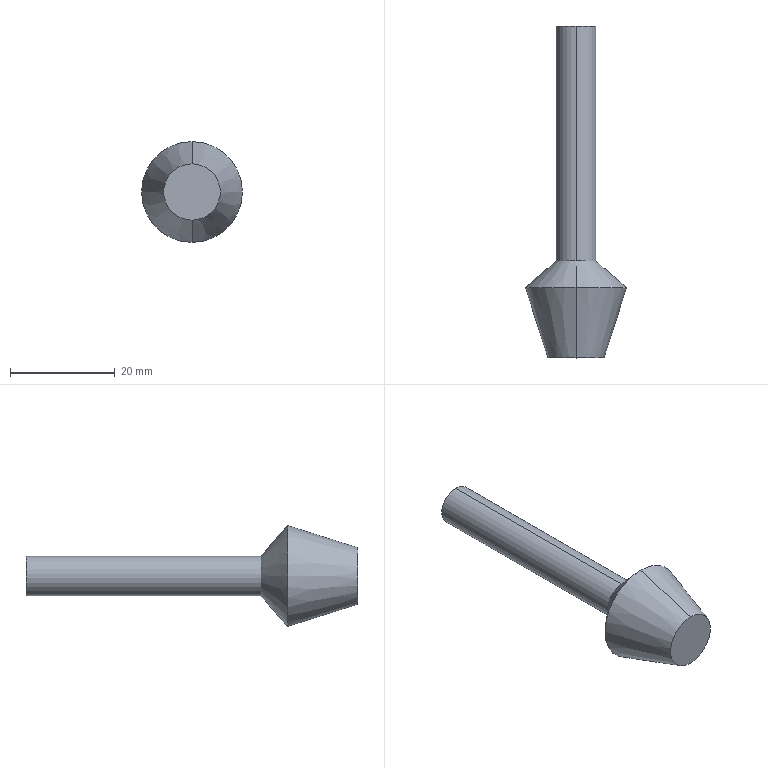Part | SolidWorks | features Revolution 1 | 1 solid | 8 faces | box 19.304 x 63.5 x 19.304 mm | volume 5277 mm3 | cone 4 | cylinder 2 | plane 2 | commonest cylinder face diameters 7.62 x2
STEP:
#1=CARTESIAN_POINT('',(0.,0.,-0.2125));
#2=VERTEX_POINT('',#1);
#3=CARTESIAN_POINT('',(0.,0.,0.2125));
#4=VERTEX_POINT('',#3);
#5=CARTESIAN_POINT('',(0.,0.,0.));
#6=DIRECTION('',(0.,-1.,0.));
#7=DIRECTION('',(0.,0.,-1.));
#8=AXIS2_PLACEMENT_3D('',#5,#6,#7);
#9=CIRCLE('',#8,0.2125);
#10=EDGE_CURVE('',#2,#4,#9,.T.);
#11=ORIENTED_EDGE('',*,*,#10,.F.);
#12=CARTESIAN_POINT('',(0.,0.53,-0.38));
#13=VERTEX_POINT('',#12);
#14=CARTESIAN_POINT('',(0.,0.53,-0.38));
#15=DIRECTION('',(0.,0.9535,-0.3013));
#16=VECTOR('',#15,39.37);
#17=LINE('',#14,#16);
#18=EDGE_CURVE('',#2,#13,#17,.T.);
#19=ORIENTED_EDGE('',*,*,#18,.T.);
#20=CARTESIAN_POINT('',(0.,0.53,0.38));
#21=VERTEX_POINT('',#20);
#22=CARTESIAN_POINT('',(0.,0.53,0.));
#23=DIRECTION('',(0.,-1.,0.));
#24=DIRECTION('',(0.,0.,-1.));
#25=AXIS2_PLACEMENT_3D('',#22,#23,#24);
#26=CIRCLE('',#25,0.38);
#27=EDGE_CURVE('',#13,#21,#26,.T.);
#28=ORIENTED_EDGE('',*,*,#27,.T.);
#29=CARTESIAN_POINT('',(0.,0.53,0.38));
#30=DIRECTION('',(0.,0.9535,0.3013));
#31=VECTOR('',#30,39.37);
#32=LINE('',#29,#31);
#33=EDGE_CURVE('',#4,#21,#32,.T.);
#34=ORIENTED_EDGE('',*,*,#33,.F.);
#35=EDGE_LOOP('',(#11,#19,#28,#34));
#36=FACE_OUTER_BOUND('',#35,.T.);
#37=CARTESIAN_POINT('',(0.,0.53,0.));
#38=DIRECTION('',(0.,1.,0.));
#39=DIRECTION('',(0.,0.,1.));
#40=AXIS2_PLACEMENT_3D('',#37,#38,#39);
#41=CONICAL_SURFACE('',#40,0.38,0.3061);
#42=ADVANCED_FACE('',(#36),#41,.T.);
#43=CARTESIAN_POINT('',(0.,2.5,-0.15));
#44=VERTEX_POINT('',#43);
#45=CARTESIAN_POINT('',(0.,2.5,0.15));
#46=VERTEX_POINT('',#45);
#47=CARTESIAN_POINT('',(0.,2.5,0.));
#48=DIRECTION('',(0.,-1.,0.));
#49=DIRECTION('',(0.,0.,-1.));
#50=AXIS2_PLACEMENT_3D('',#47,#48,#49);
#51=CIRCLE('',#50,0.15);
#52=EDGE_CURVE('',#44,#46,#51,.T.);
#53=ORIENTED_EDGE('',*,*,#52,.T.);
#54=CARTESIAN_POINT('',(0.,0.73,0.15));
#55=VERTEX_POINT('',#54);
#56=CARTESIAN_POINT('',(0.,0.,0.15));
#57=DIRECTION('',(0.,-1.,0.));
#58=VECTOR('',#57,39.37);
#59=LINE('',#56,#58);
#60=EDGE_CURVE('',#46,#55,#59,.T.);
#61=ORIENTED_EDGE('',*,*,#60,.T.);
#62=CARTESIAN_POINT('',(0.,0.73,-0.15));
#63=VERTEX_POINT('',#62);
#64=CARTESIAN_POINT('',(0.,0.73,0.));
#65=DIRECTION('',(0.,-1.,0.));
#66=DIRECTION('',(0.,0.,-1.));
#67=AXIS2_PLACEMENT_3D('',#64,#65,#66);
#68=CIRCLE('',#67,0.15);
#69=EDGE_CURVE('',#63,#55,#68,.T.);
#70=ORIENTED_EDGE('',*,*,#69,.F.);
#71=CARTESIAN_POINT('',(0.,0.,-0.15));
#72=DIRECTION('',(0.,-1.,0.));
#73=VECTOR('',#72,39.37);
#74=LINE('',#71,#73);
#75=EDGE_CURVE('',#44,#63,#74,.T.);
#76=ORIENTED_EDGE('',*,*,#75,.F.);
#77=EDGE_LOOP('',(#53,#61,#70,#76));
#78=FACE_OUTER_BOUND('',#77,.T.);
#79=CARTESIAN_POINT('',(0.,0.,0.));
#80=DIRECTION('',(0.,-1.,0.));
#81=DIRECTION('',(0.,0.,-1.));
#82=AXIS2_PLACEMENT_3D('',#79,#80,#81);
#83=CYLINDRICAL_SURFACE('',#82,0.15);
#84=ADVANCED_FACE('',(#78),#83,.T.);
#85=ORIENTED_EDGE('',*,*,#69,.T.);
#86=CARTESIAN_POINT('',(0.,0.53,0.38));
#87=DIRECTION('',(0.,-0.6562,0.7546));
#88=VECTOR('',#87,39.37);
#89=LINE('',#86,#88);
#90=EDGE_CURVE('',#55,#21,#89,.T.);
#91=ORIENTED_EDGE('',*,*,#90,.T.);
#92=ORIENTED_EDGE('',*,*,#27,.F.);
#93=CARTESIAN_POINT('',(0.,0.53,-0.38));
#94=DIRECTION('',(0.,-0.6562,-0.7546));
#95=VECTOR('',#94,39.37);
#96=LINE('',#93,#95);
#97=EDGE_CURVE('',#63,#13,#96,.T.);
#98=ORIENTED_EDGE('',*,*,#97,.F.);
#99=EDGE_LOOP('',(#85,#91,#92,#98));
#100=FACE_OUTER_BOUND('',#99,.T.);
#101=CARTESIAN_POINT('',(0.,0.53,0.));
#102=DIRECTION('',(0.,-1.,0.));
#103=DIRECTION('',(0.,0.,-1.));
#104=AXIS2_PLACEMENT_3D('',#101,#102,#103);
#105=CONICAL_SURFACE('',#104,0.38,0.8551);
#106=ADVANCED_FACE('',(#100),#105,.T.);
#107=ORIENTED_EDGE('',*,*,#90,.F.);
#108=CARTESIAN_POINT('',(0.,0.73,0.));
#109=DIRECTION('',(0.,-1.,0.));
#110=DIRECTION('',(0.,0.,-1.));
#111=AXIS2_PLACEMENT_3D('',#108,#109,#110);
#112=CIRCLE('',#111,0.15);
#113=EDGE_CURVE('',#55,#63,#112,.T.);
#114=ORIENTED_EDGE('',*,*,#113,.T.);
#115=ORIENTED_EDGE('',*,*,#97,.T.);
#116=CARTESIAN_POINT('',(0.,0.53,0.));
#117=DIRECTION('',(0.,-1.,0.));
#118=DIRECTION('',(0.,0.,-1.));
#119=AXIS2_PLACEMENT_3D('',#116,#117,#118);
#120=CIRCLE('',#119,0.38);
#121=EDGE_CURVE('',#21,#13,#120,.T.);
#122=ORIENTED_EDGE('',*,*,#121,.F.);
#123=EDGE_LOOP('',(#107,#114,#115,#122));
#124=FACE_OUTER_BOUND('',#123,.T.);
#125=CARTESIAN_POINT('',(0.,0.53,0.));
#126=DIRECTION('',(0.,-1.,0.));
#127=DIRECTION('',(0.,0.,-1.));
#128=AXIS2_PLACEMENT_3D('',#125,#126,#127);
#129=CONICAL_SURFACE('',#128,0.38,0.8551);
#130=ADVANCED_FACE('',(#124),#129,.T.);
#131=ORIENTED_EDGE('',*,*,#60,.F.);
#132=CARTESIAN_POINT('',(0.,2.5,0.));
#133=DIRECTION('',(0.,-1.,0.));
#134=DIRECTION('',(0.,0.,-1.));
#135=AXIS2_PLACEMENT_3D('',#132,#133,#134);
#136=CIRCLE('',#135,0.15);
#137=EDGE_CURVE('',#46,#44,#136,.T.);
#138=ORIENTED_EDGE('',*,*,#137,.T.);
#139=ORIENTED_EDGE('',*,*,#75,.T.);
#140=ORIENTED_EDGE('',*,*,#113,.F.);
#141=EDGE_LOOP('',(#131,#138,#139,#140));
#142=FACE_OUTER_BOUND('',#141,.T.);
#143=CARTESIAN_POINT('',(0.,0.,0.));
#144=DIRECTION('',(0.,-1.,0.));
#145=DIRECTION('',(0.,0.,-1.));
#146=AXIS2_PLACEMENT_3D('',#143,#144,#145);
#147=CYLINDRICAL_SURFACE('',#146,0.15);
#148=ADVANCED_FACE('',(#142),#147,.T.);
#149=ORIENTED_EDGE('',*,*,#52,.F.);
#150=ORIENTED_EDGE('',*,*,#137,.F.);
#151=EDGE_LOOP('',(#149,#150));
#152=FACE_OUTER_BOUND('',#151,.T.);
#153=CARTESIAN_POINT('',(0.,2.5,0.));
#154=DIRECTION('',(0.,-1.,0.));
#155=DIRECTION('',(0.,0.,-1.));
#156=AXIS2_PLACEMENT_3D('',#153,#154,#155);
#157=PLANE('',#156);
#158=ADVANCED_FACE('',(#152),#157,.F.);
#159=CARTESIAN_POINT('',(0.,0.,0.));
#160=DIRECTION('',(0.,-1.,0.));
#161=DIRECTION('',(0.,0.,-1.));
#162=AXIS2_PLACEMENT_3D('',#159,#160,#161);
#163=CIRCLE('',#162,0.2125);
#164=EDGE_CURVE('',#4,#2,#163,.T.);
#165=ORIENTED_EDGE('',*,*,#164,.T.);
#166=ORIENTED_EDGE('',*,*,#10,.T.);
#167=EDGE_LOOP('',(#165,#166));
#168=FACE_OUTER_BOUND('',#167,.T.);
#169=CARTESIAN_POINT('',(0.,0.,0.));
#170=DIRECTION('',(0.,-1.,0.));
#171=DIRECTION('',(0.,0.,-1.));
#172=AXIS2_PLACEMENT_3D('',#169,#170,#171);
#173=PLANE('',#172);
#174=ADVANCED_FACE('',(#168),#173,.T.);
#175=ORIENTED_EDGE('',*,*,#18,.F.);
#176=ORIENTED_EDGE('',*,*,#164,.F.);
#177=ORIENTED_EDGE('',*,*,#33,.T.);
#178=ORIENTED_EDGE('',*,*,#121,.T.);
#179=EDGE_LOOP('',(#175,#176,#177,#178));
#180=FACE_OUTER_BOUND('',#179,.T.);
#181=CARTESIAN_POINT('',(0.,0.53,0.));
#182=DIRECTION('',(0.,1.,0.));
#183=DIRECTION('',(0.,0.,1.));
#184=AXIS2_PLACEMENT_3D('',#181,#182,#183);
#185=CONICAL_SURFACE('',#184,0.38,0.3061);
#186=ADVANCED_FACE('',(#180),#185,.T.);
#187=CLOSED_SHELL('',(#42,#84,#106,#130,#148,#158,#174,#186));
#188=MANIFOLD_SOLID_BREP('',#187);
#189=CARTESIAN_POINT('',(0.,0.,0.));
#190=DIRECTION('',(0.,0.,1.));
#191=DIRECTION('',(1.,0.,0.));
#192=AXIS2_PLACEMENT_3D('',#189,#190,#191);
#193=(LENGTH_UNIT()NAMED_UNIT(*)SI_UNIT($,.METRE.));
#194=LENGTH_MEASURE_WITH_UNIT(LENGTH_MEASURE(0.0254),#193);
#195=DIMENSIONAL_EXPONENTS(1.,0.,0.,0.,0.,0.,0.);
#196=(CONVERSION_BASED_UNIT('INCH',#194)LENGTH_UNIT()NAMED_UNIT(#195));
#197=UNCERTAINTY_MEASURE_WITH_UNIT(LENGTH_MEASURE(0.00001),#196,'','');
#198=(NAMED_UNIT(*)PLANE_ANGLE_UNIT()SI_UNIT($,.RADIAN.));
#199=(NAMED_UNIT(*)SI_UNIT($,.STERADIAN.)SOLID_ANGLE_UNIT());
#200=(GEOMETRIC_REPRESENTATION_CONTEXT(3)GLOBAL_UNCERTAINTY_ASSIGNED_CONTEXT((#197))GLOBAL_UNIT_ASSIGNED_CONTEXT((#196,#198,#199))REPRESENTATION_CONTEXT('',''));
#201=ADVANCED_BREP_SHAPE_REPRESENTATION('',(#188,#192),#200);